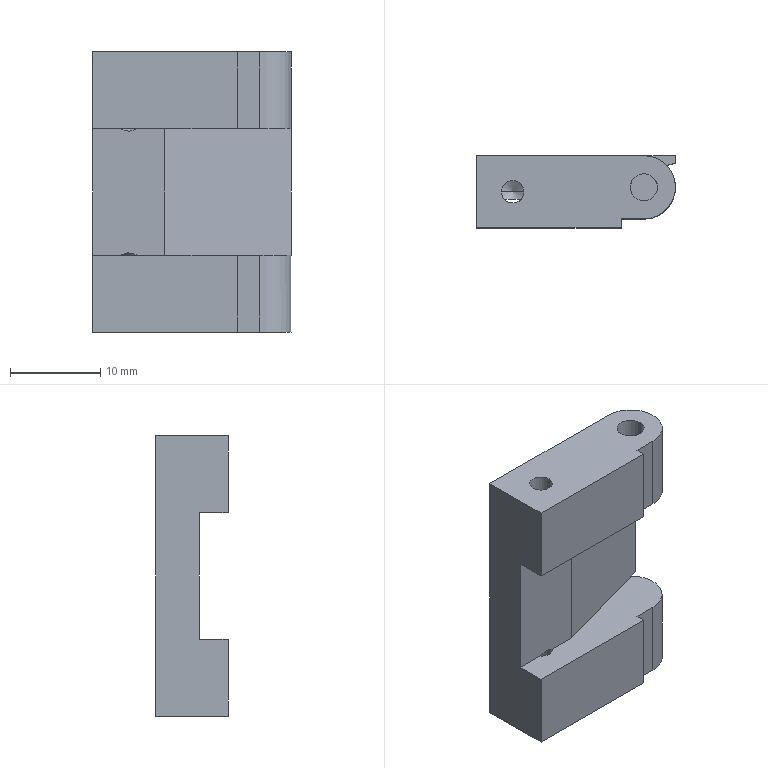Part | STEP file | PN_0022 Mount electronic clip pressure block | 1 solid | 34 faces | box 22 x 8 x 31 mm | volume 3731 mm3 | plane 19 | cylinder 11 | cone 4 | commonest cylinder face diameters 2.5 x4 3 x4 7 x3